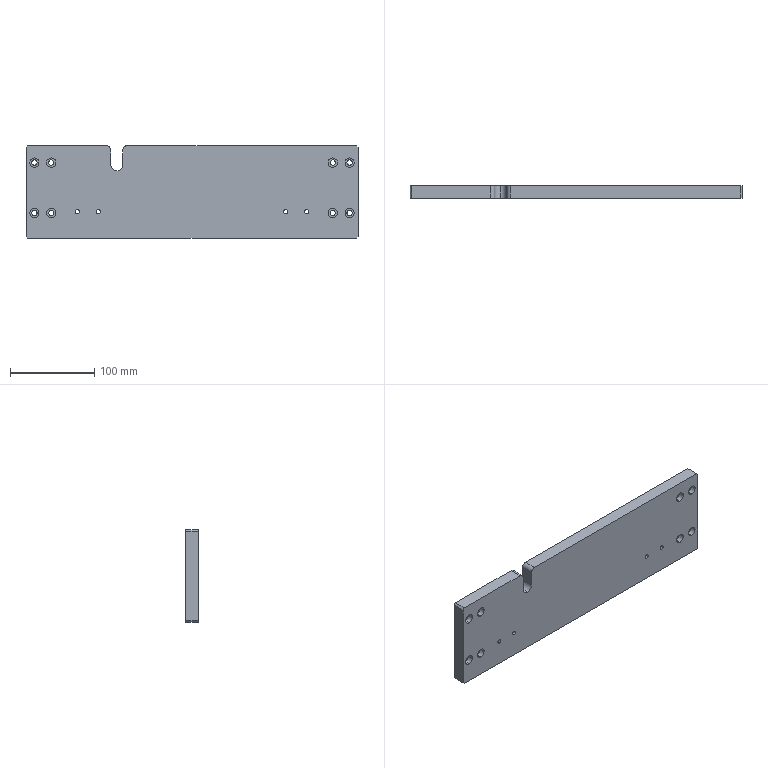Part | SolidWorks | features BaseBody 1 | 1 solid | 65 faces | box 395 x 15 x 110 mm | volume 637026 mm3 | cylinder 44 | plane 21 | commonest cylinder face diameters 6.4 x16 11 x16 5 x8 10 x2 14 x2